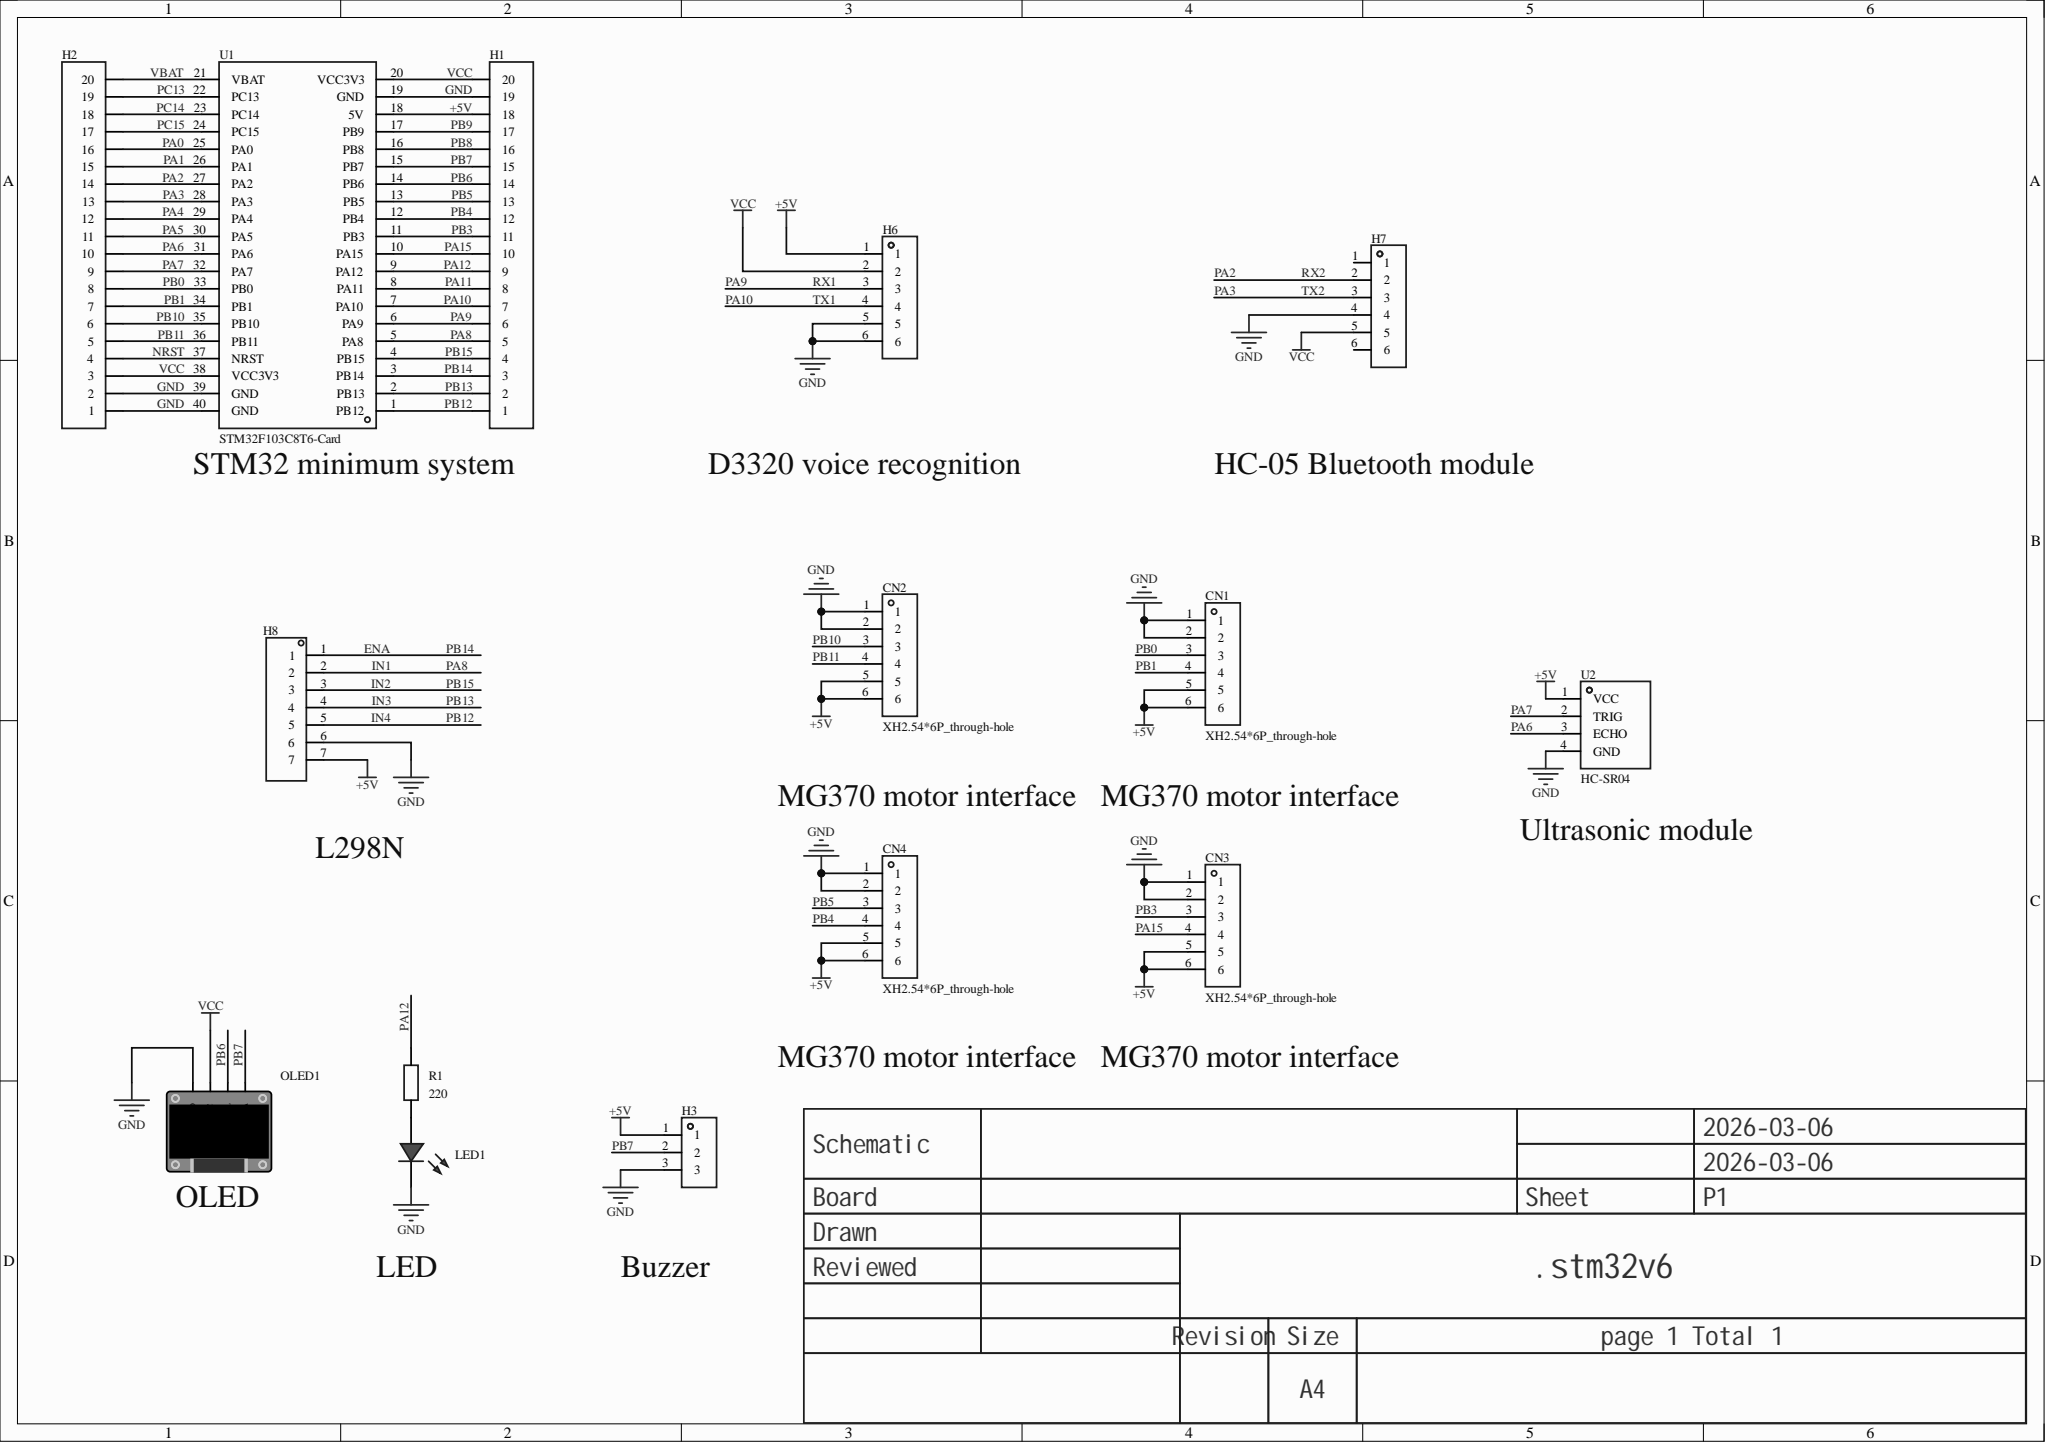Circuit board | Altium Designer | 15 parts | 38 nets
Bill of materials:
Comment,Description,Designator,Footprint,LibRef,Quantity
"XH2.54*6P_through-hole","","CN1, CN2, CN3, CN4","CONN-TH_XH2.54-6P","XH2.54*6P_直插","4"
"","","H1, H2","HDR-TH_20P-P2.54-V-F","HDR-F_2.54_1x20P","2"
"","","H3","HDR-TH_3P-P2.54-V-F","HDR-F_2.54_1x3P","1"
"","","H6, H7","HDR-TH_6P-P2.54-V-F","HDR-F_2.54_1x6P","2"
"","","H8","HDR-TH_7P-P2.54-V-F","HDR-F_2.54_1x7P","1"
"","","LED1","LED_TH-3mm","LED_TH-R_3mm","1"
"","","OLED1","0.96OLED_4P","0.96OLED模块_4P","1"
"220","","R1","R0603","Res_0603","1"
"STM32F103C8T6-Card","","U1","CONN-TH_L53.3-W22.9_STM32F103C8T6-CARD","STM32F103C8T6-Card","1"
"HC-SR04","","U2","TH_HC-SR04V","HC-SR04","1"
Netlist (Protel format):
[
CN1
CONN-TH_XH2.54-6P
XH2.54*6P_through-hole



]
[
CN2
CONN-TH_XH2.54-6P
XH2.54*6P_through-hole



]
[
CN3
CONN-TH_XH2.54-6P
XH2.54*6P_through-hole



]
[
CN4
CONN-TH_XH2.54-6P
XH2.54*6P_through-hole



]
[
H1
HDR-TH_20P-P2.54-V-F




]
[
H2
HDR-TH_20P-P2.54-V-F




]
[
H3
HDR-TH_3P-P2.54-V-F




]
[
H6
HDR-TH_6P-P2.54-V-F




]
[
H7
HDR-TH_6P-P2.54-V-F




]
[
H8
HDR-TH_7P-P2.54-V-F




]
[
LED1
LED_TH-3mm




]
[
OLED1
0.96OLED_4P




]
[
R1
R0603
220



]
[
U1
CONN-TH_L53.3-W22.9_STM32F103C8T6-CARD
STM32F103C8T6-Card



]
[
U2
TH_HC-SR04V
HC-SR04



]
(
VCC
H1-20
H2-3
H6-2
H7-5
OLED1-2
U1-20
U1-38
)
(
VBAT
H2-20
U1-21
)
(
PC15
H2-17
U1-24
)
(
PC14
H2-18
U1-23
)
(
PC13
H2-19
U1-22
)
(
PB11
CN2-4
H2-5
U1-36
)
(
PB10
CN2-3
H2-6
U1-35
)
(
PB9
H1-17
U1-17
)
(
PB8
H1-16
U1-16
)
(
PB7
H1-15
H3-2
OLED1-4
U1-15
)
(
PB6
H1-14
OLED1-3
U1-14
)
(
PB5
CN4-3
H1-13
U1-13
)
(
PB4
CN4-4
H1-12
U1-12
)
(
PB3
CN3-3
H1-11
U1-11
)
(
PB1
CN1-4
H2-7
U1-34
)
(
PB0
CN1-3
H2-8
U1-33
)
(
PA15
CN3-4
H1-10
U1-10
)
(
PA12
H1-9
R1-2
U1-9
)
(
PA11
H1-8
U1-8
)
(
PA10
H1-7
H6-4
U1-7
)
(
PA9
H1-6
H6-3
U1-6
)
(
PA7
H2-9
U1-32
U2-2
)
(
PA6
H2-10
U1-31
U2-3
)
(
PA5
H2-11
U1-30
)
(
PA4
H2-12
U1-29
)
(
PA3
H2-13
H7-3
U1-28
)
(
PA2
H2-14
H7-2
U1-27
)
(
PA1
H2-15
U1-26
)
(
PA0
H2-16
U1-25
)
(
NRST
H2-4
U1-37
)
(
NetLED1_1
LED1-1
R1-1
)
(
IN4
H1-1
H8-5
U1-1
)
(
IN3
H1-2
H8-4
U1-2
)
(
IN2
H1-4
H8-3
U1-4
)
(
IN1
H1-5
H8-2
U1-5
)
(
GND
CN1-1
CN1-2
CN2-1
CN2-2
CN3-1
CN3-2
CN4-1
CN4-2
H1-19
H2-1
H2-2
H3-3
H6-5
H6-6
H7-4
H8-6
LED1-2
OLED1-1
U1-19
U1-39
U1-40
U2-4
)
(
ENA
H1-3
H8-1
U1-3
)
(
+5V
CN1-5
CN1-6
CN2-5
CN2-6
CN3-5
CN3-6
CN4-5
CN4-6
H1-18
H3-1
H6-1
H8-7
U1-18
U2-1
)